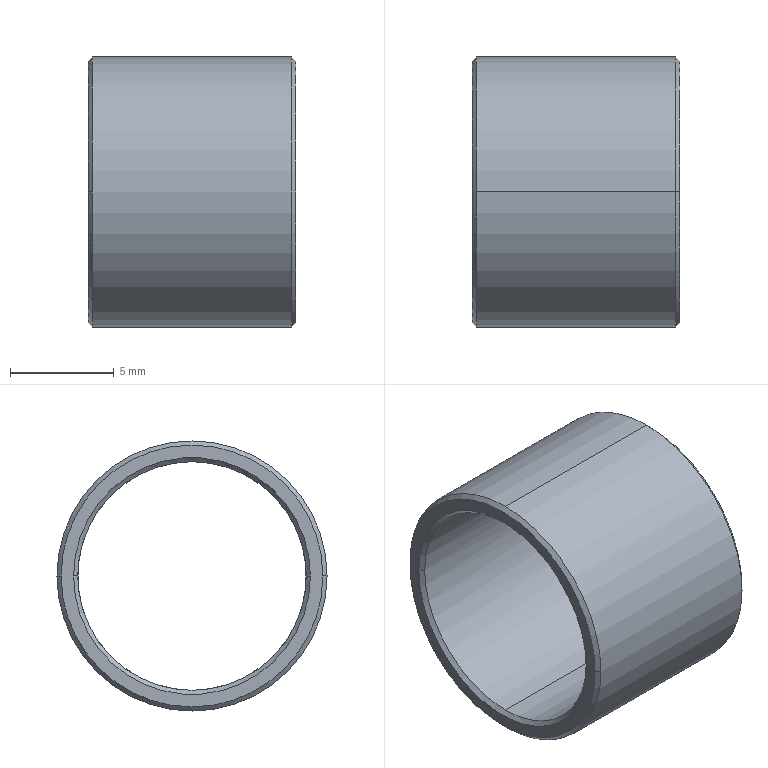Part | SolidWorks | features BaseBody 1 | 1 solid | 14 faces | box 10 x 13 x 13 mm | volume 373.975 mm3 | cone 8 | cylinder 4 | plane 2 | commonest cylinder face diameters 11 x2 13 x2
STEP:
#1=CARTESIAN_POINT('',(9.8,0.,6.5));
#2=VERTEX_POINT('',#1);
#3=CARTESIAN_POINT('',(9.8,0.,-6.5));
#4=VERTEX_POINT('',#3);
#5=CARTESIAN_POINT('',(9.8,0.,0.));
#6=DIRECTION('',(-1.,0.,0.));
#7=DIRECTION('',(0.,0.,1.));
#8=AXIS2_PLACEMENT_3D('',#5,#6,#7);
#9=CIRCLE('',#8,6.5);
#10=EDGE_CURVE('',#2,#4,#9,.T.);
#11=ORIENTED_EDGE('',*,*,#10,.T.);
#12=CARTESIAN_POINT('',(0.2,0.,-6.5));
#13=VERTEX_POINT('',#12);
#14=CARTESIAN_POINT('',(5.,0.,-6.5));
#15=DIRECTION('',(-1.,0.,0.));
#16=VECTOR('',#15,1000.);
#17=LINE('',#14,#16);
#18=EDGE_CURVE('',#4,#13,#17,.T.);
#19=ORIENTED_EDGE('',*,*,#18,.T.);
#20=CARTESIAN_POINT('',(0.2,6.5,0.));
#21=VERTEX_POINT('',#20);
#22=CARTESIAN_POINT('',(0.2,0.,0.));
#23=DIRECTION('',(1.,0.,0.));
#24=DIRECTION('',(0.,0.,1.));
#25=AXIS2_PLACEMENT_3D('',#22,#23,#24);
#26=CIRCLE('',#25,6.5);
#27=EDGE_CURVE('',#13,#21,#26,.T.);
#28=ORIENTED_EDGE('',*,*,#27,.T.);
#29=CARTESIAN_POINT('',(0.2,0.,6.5));
#30=VERTEX_POINT('',#29);
#31=CARTESIAN_POINT('',(0.2,0.,0.));
#32=DIRECTION('',(1.,0.,0.));
#33=DIRECTION('',(0.,0.,1.));
#34=AXIS2_PLACEMENT_3D('',#31,#32,#33);
#35=CIRCLE('',#34,6.5);
#36=EDGE_CURVE('',#21,#30,#35,.T.);
#37=ORIENTED_EDGE('',*,*,#36,.T.);
#38=CARTESIAN_POINT('',(5.,0.,6.5));
#39=DIRECTION('',(-1.,0.,0.));
#40=VECTOR('',#39,1000.);
#41=LINE('',#38,#40);
#42=EDGE_CURVE('',#2,#30,#41,.T.);
#43=ORIENTED_EDGE('',*,*,#42,.F.);
#44=EDGE_LOOP('',(#11,#19,#28,#37,#43));
#45=FACE_OUTER_BOUND('',#44,.T.);
#46=CARTESIAN_POINT('',(5.,0.,0.));
#47=DIRECTION('',(-1.,0.,0.));
#48=DIRECTION('',(0.,0.,1.));
#49=AXIS2_PLACEMENT_3D('',#46,#47,#48);
#50=CYLINDRICAL_SURFACE('',#49,6.5);
#51=ADVANCED_FACE('',(#45),#50,.T.);
#52=CARTESIAN_POINT('',(10.,0.,6.3));
#53=VERTEX_POINT('',#52);
#54=CARTESIAN_POINT('',(10.,0.,-6.3));
#55=VERTEX_POINT('',#54);
#56=CARTESIAN_POINT('',(10.,0.,0.));
#57=DIRECTION('',(-1.,0.,0.));
#58=DIRECTION('',(0.,0.,1.));
#59=AXIS2_PLACEMENT_3D('',#56,#57,#58);
#60=CIRCLE('',#59,6.3);
#61=EDGE_CURVE('',#53,#55,#60,.T.);
#62=ORIENTED_EDGE('',*,*,#61,.T.);
#63=CARTESIAN_POINT('',(9.8,0.,-6.5));
#64=DIRECTION('',(-0.7071,0.,-0.7071));
#65=VECTOR('',#64,1000.);
#66=LINE('',#63,#65);
#67=EDGE_CURVE('',#55,#4,#66,.T.);
#68=ORIENTED_EDGE('',*,*,#67,.T.);
#69=ORIENTED_EDGE('',*,*,#10,.F.);
#70=CARTESIAN_POINT('',(9.8,0.,6.5));
#71=DIRECTION('',(-0.7071,0.,0.7071));
#72=VECTOR('',#71,1000.);
#73=LINE('',#70,#72);
#74=EDGE_CURVE('',#53,#2,#73,.T.);
#75=ORIENTED_EDGE('',*,*,#74,.F.);
#76=EDGE_LOOP('',(#62,#68,#69,#75));
#77=FACE_OUTER_BOUND('',#76,.T.);
#78=CARTESIAN_POINT('',(9.8,0.,0.));
#79=DIRECTION('',(-1.,0.,0.));
#80=DIRECTION('',(0.,0.,1.));
#81=AXIS2_PLACEMENT_3D('',#78,#79,#80);
#82=CONICAL_SURFACE('',#81,6.5,0.7854);
#83=ADVANCED_FACE('',(#77),#82,.T.);
#84=CARTESIAN_POINT('',(0.,6.3,0.));
#85=VERTEX_POINT('',#84);
#86=CARTESIAN_POINT('',(0.,-6.3,0.));
#87=VERTEX_POINT('',#86);
#88=CARTESIAN_POINT('',(0.,0.,0.));
#89=DIRECTION('',(1.,0.,0.));
#90=DIRECTION('',(0.,1.,0.));
#91=AXIS2_PLACEMENT_3D('',#88,#89,#90);
#92=CIRCLE('',#91,6.3);
#93=EDGE_CURVE('',#85,#87,#92,.T.);
#94=ORIENTED_EDGE('',*,*,#93,.T.);
#95=CARTESIAN_POINT('',(0.2,-6.5,0.));
#96=VERTEX_POINT('',#95);
#97=CARTESIAN_POINT('',(0.2,-6.5,0.));
#98=DIRECTION('',(0.7071,-0.7071,0.));
#99=VECTOR('',#98,1000.);
#100=LINE('',#97,#99);
#101=EDGE_CURVE('',#87,#96,#100,.T.);
#102=ORIENTED_EDGE('',*,*,#101,.T.);
#103=CARTESIAN_POINT('',(0.2,0.,0.));
#104=DIRECTION('',(1.,0.,0.));
#105=DIRECTION('',(0.,0.,1.));
#106=AXIS2_PLACEMENT_3D('',#103,#104,#105);
#107=CIRCLE('',#106,6.5);
#108=EDGE_CURVE('',#30,#96,#107,.T.);
#109=ORIENTED_EDGE('',*,*,#108,.F.);
#110=ORIENTED_EDGE('',*,*,#36,.F.);
#111=CARTESIAN_POINT('',(0.2,6.5,0.));
#112=DIRECTION('',(0.7071,0.7071,0.));
#113=VECTOR('',#112,1000.);
#114=LINE('',#111,#113);
#115=EDGE_CURVE('',#85,#21,#114,.T.);
#116=ORIENTED_EDGE('',*,*,#115,.F.);
#117=EDGE_LOOP('',(#94,#102,#109,#110,#116));
#118=FACE_OUTER_BOUND('',#117,.T.);
#119=CARTESIAN_POINT('',(0.2,0.,0.));
#120=DIRECTION('',(1.,0.,0.));
#121=DIRECTION('',(0.,1.,0.));
#122=AXIS2_PLACEMENT_3D('',#119,#120,#121);
#123=CONICAL_SURFACE('',#122,6.5,0.7854);
#124=ADVANCED_FACE('',(#118),#123,.T.);
#125=CARTESIAN_POINT('',(9.8,0.,5.5));
#126=VERTEX_POINT('',#125);
#127=CARTESIAN_POINT('',(9.8,0.,-5.5));
#128=VERTEX_POINT('',#127);
#129=CARTESIAN_POINT('',(9.8,0.,0.));
#130=DIRECTION('',(1.,0.,0.));
#131=DIRECTION('',(0.,-1.,0.));
#132=AXIS2_PLACEMENT_3D('',#129,#130,#131);
#133=CIRCLE('',#132,5.5);
#134=EDGE_CURVE('',#126,#128,#133,.T.);
#135=ORIENTED_EDGE('',*,*,#134,.F.);
#136=CARTESIAN_POINT('',(10.,0.,5.7));
#137=VERTEX_POINT('',#136);
#138=CARTESIAN_POINT('',(10.,0.,5.7));
#139=DIRECTION('',(0.7071,0.,0.7071));
#140=VECTOR('',#139,1000.);
#141=LINE('',#138,#140);
#142=EDGE_CURVE('',#126,#137,#141,.T.);
#143=ORIENTED_EDGE('',*,*,#142,.T.);
#144=CARTESIAN_POINT('',(10.,0.,-5.7));
#145=VERTEX_POINT('',#144);
#146=CARTESIAN_POINT('',(10.,0.,0.));
#147=DIRECTION('',(-1.,0.,0.));
#148=DIRECTION('',(0.,0.,-1.));
#149=AXIS2_PLACEMENT_3D('',#146,#147,#148);
#150=CIRCLE('',#149,5.7);
#151=EDGE_CURVE('',#145,#137,#150,.T.);
#152=ORIENTED_EDGE('',*,*,#151,.F.);
#153=CARTESIAN_POINT('',(10.,0.,-5.7));
#154=DIRECTION('',(0.7071,0.,-0.7071));
#155=VECTOR('',#154,1000.);
#156=LINE('',#153,#155);
#157=EDGE_CURVE('',#128,#145,#156,.T.);
#158=ORIENTED_EDGE('',*,*,#157,.F.);
#159=EDGE_LOOP('',(#135,#143,#152,#158));
#160=FACE_OUTER_BOUND('',#159,.T.);
#161=CARTESIAN_POINT('',(10.,0.,0.));
#162=DIRECTION('',(1.,0.,0.));
#163=DIRECTION('',(0.,0.,-1.));
#164=AXIS2_PLACEMENT_3D('',#161,#162,#163);
#165=CONICAL_SURFACE('',#164,5.7,0.7854);
#166=ADVANCED_FACE('',(#160),#165,.F.);
#167=CARTESIAN_POINT('',(0.2,5.5,0.));
#168=VERTEX_POINT('',#167);
#169=CARTESIAN_POINT('',(0.2,0.,-5.5));
#170=VERTEX_POINT('',#169);
#171=CARTESIAN_POINT('',(0.2,0.,0.));
#172=DIRECTION('',(-1.,0.,0.));
#173=DIRECTION('',(0.,-1.,0.));
#174=AXIS2_PLACEMENT_3D('',#171,#172,#173);
#175=CIRCLE('',#174,5.5);
#176=EDGE_CURVE('',#168,#170,#175,.T.);
#177=ORIENTED_EDGE('',*,*,#176,.F.);
#178=CARTESIAN_POINT('',(0.,5.7,0.));
#179=VERTEX_POINT('',#178);
#180=CARTESIAN_POINT('',(0.,5.7,0.));
#181=DIRECTION('',(-0.7071,0.7071,0.));
#182=VECTOR('',#181,1000.);
#183=LINE('',#180,#182);
#184=EDGE_CURVE('',#168,#179,#183,.T.);
#185=ORIENTED_EDGE('',*,*,#184,.T.);
#186=CARTESIAN_POINT('',(0.,-5.7,0.));
#187=VERTEX_POINT('',#186);
#188=CARTESIAN_POINT('',(0.,0.,0.));
#189=DIRECTION('',(1.,0.,0.));
#190=DIRECTION('',(0.,-1.,0.));
#191=AXIS2_PLACEMENT_3D('',#188,#189,#190);
#192=CIRCLE('',#191,5.7);
#193=EDGE_CURVE('',#187,#179,#192,.T.);
#194=ORIENTED_EDGE('',*,*,#193,.F.);
#195=CARTESIAN_POINT('',(0.2,-5.5,0.));
#196=VERTEX_POINT('',#195);
#197=CARTESIAN_POINT('',(0.,-5.7,0.));
#198=DIRECTION('',(-0.7071,-0.7071,0.));
#199=VECTOR('',#198,1000.);
#200=LINE('',#197,#199);
#201=EDGE_CURVE('',#196,#187,#200,.T.);
#202=ORIENTED_EDGE('',*,*,#201,.F.);
#203=CARTESIAN_POINT('',(0.2,0.,0.));
#204=DIRECTION('',(-1.,0.,0.));
#205=DIRECTION('',(0.,-1.,0.));
#206=AXIS2_PLACEMENT_3D('',#203,#204,#205);
#207=CIRCLE('',#206,5.5);
#208=EDGE_CURVE('',#170,#196,#207,.T.);
#209=ORIENTED_EDGE('',*,*,#208,.F.);
#210=EDGE_LOOP('',(#177,#185,#194,#202,#209));
#211=FACE_OUTER_BOUND('',#210,.T.);
#212=CARTESIAN_POINT('',(0.,0.,0.));
#213=DIRECTION('',(-1.,0.,0.));
#214=DIRECTION('',(0.,-1.,0.));
#215=AXIS2_PLACEMENT_3D('',#212,#213,#214);
#216=CONICAL_SURFACE('',#215,5.7,0.7854);
#217=ADVANCED_FACE('',(#211),#216,.F.);
#218=ORIENTED_EDGE('',*,*,#134,.T.);
#219=CARTESIAN_POINT('',(5.,0.,-5.5));
#220=DIRECTION('',(-1.,0.,0.));
#221=VECTOR('',#220,1000.);
#222=LINE('',#219,#221);
#223=EDGE_CURVE('',#128,#170,#222,.T.);
#224=ORIENTED_EDGE('',*,*,#223,.T.);
#225=ORIENTED_EDGE('',*,*,#208,.T.);
#226=CARTESIAN_POINT('',(0.2,0.,5.5));
#227=VERTEX_POINT('',#226);
#228=CARTESIAN_POINT('',(0.2,0.,0.));
#229=DIRECTION('',(-1.,0.,0.));
#230=DIRECTION('',(0.,-1.,0.));
#231=AXIS2_PLACEMENT_3D('',#228,#229,#230);
#232=CIRCLE('',#231,5.5);
#233=EDGE_CURVE('',#196,#227,#232,.T.);
#234=ORIENTED_EDGE('',*,*,#233,.T.);
#235=CARTESIAN_POINT('',(5.,0.,5.5));
#236=DIRECTION('',(-1.,0.,0.));
#237=VECTOR('',#236,1000.);
#238=LINE('',#235,#237);
#239=EDGE_CURVE('',#126,#227,#238,.T.);
#240=ORIENTED_EDGE('',*,*,#239,.F.);
#241=EDGE_LOOP('',(#218,#224,#225,#234,#240));
#242=FACE_OUTER_BOUND('',#241,.T.);
#243=CARTESIAN_POINT('',(5.,0.,0.));
#244=DIRECTION('',(-1.,0.,0.));
#245=DIRECTION('',(0.,0.,1.));
#246=AXIS2_PLACEMENT_3D('',#243,#244,#245);
#247=CYLINDRICAL_SURFACE('',#246,5.5);
#248=ADVANCED_FACE('',(#242),#247,.F.);
#249=ORIENTED_EDGE('',*,*,#18,.F.);
#250=CARTESIAN_POINT('',(9.8,0.,0.));
#251=DIRECTION('',(-1.,0.,0.));
#252=DIRECTION('',(0.,0.,1.));
#253=AXIS2_PLACEMENT_3D('',#250,#251,#252);
#254=CIRCLE('',#253,6.5);
#255=EDGE_CURVE('',#4,#2,#254,.T.);
#256=ORIENTED_EDGE('',*,*,#255,.T.);
#257=ORIENTED_EDGE('',*,*,#42,.T.);
#258=ORIENTED_EDGE('',*,*,#108,.T.);
#259=CARTESIAN_POINT('',(0.2,0.,0.));
#260=DIRECTION('',(1.,0.,0.));
#261=DIRECTION('',(0.,0.,1.));
#262=AXIS2_PLACEMENT_3D('',#259,#260,#261);
#263=CIRCLE('',#262,6.5);
#264=EDGE_CURVE('',#96,#13,#263,.T.);
#265=ORIENTED_EDGE('',*,*,#264,.T.);
#266=EDGE_LOOP('',(#249,#256,#257,#258,#265));
#267=FACE_OUTER_BOUND('',#266,.T.);
#268=CARTESIAN_POINT('',(5.,0.,0.));
#269=DIRECTION('',(-1.,0.,0.));
#270=DIRECTION('',(0.,0.,1.));
#271=AXIS2_PLACEMENT_3D('',#268,#269,#270);
#272=CYLINDRICAL_SURFACE('',#271,6.5);
#273=ADVANCED_FACE('',(#267),#272,.T.);
#274=ORIENTED_EDGE('',*,*,#67,.F.);
#275=CARTESIAN_POINT('',(10.,0.,0.));
#276=DIRECTION('',(-1.,0.,0.));
#277=DIRECTION('',(0.,0.,1.));
#278=AXIS2_PLACEMENT_3D('',#275,#276,#277);
#279=CIRCLE('',#278,6.3);
#280=EDGE_CURVE('',#55,#53,#279,.T.);
#281=ORIENTED_EDGE('',*,*,#280,.T.);
#282=ORIENTED_EDGE('',*,*,#74,.T.);
#283=ORIENTED_EDGE('',*,*,#255,.F.);
#284=EDGE_LOOP('',(#274,#281,#282,#283));
#285=FACE_OUTER_BOUND('',#284,.T.);
#286=CARTESIAN_POINT('',(9.8,0.,0.));
#287=DIRECTION('',(-1.,0.,0.));
#288=DIRECTION('',(0.,0.,1.));
#289=AXIS2_PLACEMENT_3D('',#286,#287,#288);
#290=CONICAL_SURFACE('',#289,6.5,0.7854);
#291=ADVANCED_FACE('',(#285),#290,.T.);
#292=ORIENTED_EDGE('',*,*,#101,.F.);
#293=CARTESIAN_POINT('',(0.,0.,0.));
#294=DIRECTION('',(1.,0.,0.));
#295=DIRECTION('',(0.,1.,0.));
#296=AXIS2_PLACEMENT_3D('',#293,#294,#295);
#297=CIRCLE('',#296,6.3);
#298=EDGE_CURVE('',#87,#85,#297,.T.);
#299=ORIENTED_EDGE('',*,*,#298,.T.);
#300=ORIENTED_EDGE('',*,*,#115,.T.);
#301=ORIENTED_EDGE('',*,*,#27,.F.);
#302=ORIENTED_EDGE('',*,*,#264,.F.);
#303=EDGE_LOOP('',(#292,#299,#300,#301,#302));
#304=FACE_OUTER_BOUND('',#303,.T.);
#305=CARTESIAN_POINT('',(0.2,0.,0.));
#306=DIRECTION('',(1.,0.,0.));
#307=DIRECTION('',(0.,1.,0.));
#308=AXIS2_PLACEMENT_3D('',#305,#306,#307);
#309=CONICAL_SURFACE('',#308,6.5,0.7854);
#310=ADVANCED_FACE('',(#304),#309,.T.);
#311=ORIENTED_EDGE('',*,*,#151,.T.);
#312=CARTESIAN_POINT('',(10.,0.,0.));
#313=DIRECTION('',(-1.,0.,0.));
#314=DIRECTION('',(0.,0.,-1.));
#315=AXIS2_PLACEMENT_3D('',#312,#313,#314);
#316=CIRCLE('',#315,5.7);
#317=EDGE_CURVE('',#137,#145,#316,.T.);
#318=ORIENTED_EDGE('',*,*,#317,.T.);
#319=EDGE_LOOP('',(#311,#318));
#320=FACE_BOUND('',#319,.T.);
#321=ORIENTED_EDGE('',*,*,#61,.F.);
#322=ORIENTED_EDGE('',*,*,#280,.F.);
#323=EDGE_LOOP('',(#321,#322));
#324=FACE_OUTER_BOUND('',#323,.T.);
#325=CARTESIAN_POINT('',(10.,-3.25,0.));
#326=DIRECTION('',(1.,0.,0.));
#327=DIRECTION('',(0.,0.,-1.));
#328=AXIS2_PLACEMENT_3D('',#325,#326,#327);
#329=PLANE('',#328);
#330=ADVANCED_FACE('',(#320,#324),#329,.T.);
#331=ORIENTED_EDGE('',*,*,#93,.F.);
#332=ORIENTED_EDGE('',*,*,#298,.F.);
#333=EDGE_LOOP('',(#331,#332));
#334=FACE_OUTER_BOUND('',#333,.T.);
#335=ORIENTED_EDGE('',*,*,#193,.T.);
#336=CARTESIAN_POINT('',(0.,0.,0.));
#337=DIRECTION('',(1.,0.,0.));
#338=DIRECTION('',(0.,-1.,0.));
#339=AXIS2_PLACEMENT_3D('',#336,#337,#338);
#340=CIRCLE('',#339,5.7);
#341=EDGE_CURVE('',#179,#187,#340,.T.);
#342=ORIENTED_EDGE('',*,*,#341,.T.);
#343=EDGE_LOOP('',(#335,#342));
#344=FACE_BOUND('',#343,.T.);
#345=CARTESIAN_POINT('',(0.,-3.25,0.));
#346=DIRECTION('',(-1.,0.,0.));
#347=DIRECTION('',(0.,0.,1.));
#348=AXIS2_PLACEMENT_3D('',#345,#346,#347);
#349=PLANE('',#348);
#350=ADVANCED_FACE('',(#334,#344),#349,.T.);
#351=ORIENTED_EDGE('',*,*,#142,.F.);
#352=CARTESIAN_POINT('',(9.8,0.,0.));
#353=DIRECTION('',(1.,0.,0.));
#354=DIRECTION('',(0.,-1.,0.));
#355=AXIS2_PLACEMENT_3D('',#352,#353,#354);
#356=CIRCLE('',#355,5.5);
#357=EDGE_CURVE('',#128,#126,#356,.T.);
#358=ORIENTED_EDGE('',*,*,#357,.F.);
#359=ORIENTED_EDGE('',*,*,#157,.T.);
#360=ORIENTED_EDGE('',*,*,#317,.F.);
#361=EDGE_LOOP('',(#351,#358,#359,#360));
#362=FACE_OUTER_BOUND('',#361,.T.);
#363=CARTESIAN_POINT('',(10.,0.,0.));
#364=DIRECTION('',(1.,0.,0.));
#365=DIRECTION('',(0.,0.,-1.));
#366=AXIS2_PLACEMENT_3D('',#363,#364,#365);
#367=CONICAL_SURFACE('',#366,5.7,0.7854);
#368=ADVANCED_FACE('',(#362),#367,.F.);
#369=ORIENTED_EDGE('',*,*,#184,.F.);
#370=CARTESIAN_POINT('',(0.2,0.,0.));
#371=DIRECTION('',(-1.,0.,0.));
#372=DIRECTION('',(0.,-1.,0.));
#373=AXIS2_PLACEMENT_3D('',#370,#371,#372);
#374=CIRCLE('',#373,5.5);
#375=EDGE_CURVE('',#227,#168,#374,.T.);
#376=ORIENTED_EDGE('',*,*,#375,.F.);
#377=ORIENTED_EDGE('',*,*,#233,.F.);
#378=ORIENTED_EDGE('',*,*,#201,.T.);
#379=ORIENTED_EDGE('',*,*,#341,.F.);
#380=EDGE_LOOP('',(#369,#376,#377,#378,#379));
#381=FACE_OUTER_BOUND('',#380,.T.);
#382=CARTESIAN_POINT('',(0.,0.,0.));
#383=DIRECTION('',(-1.,0.,0.));
#384=DIRECTION('',(0.,-1.,0.));
#385=AXIS2_PLACEMENT_3D('',#382,#383,#384);
#386=CONICAL_SURFACE('',#385,5.7,0.7854);
#387=ADVANCED_FACE('',(#381),#386,.F.);
#388=ORIENTED_EDGE('',*,*,#223,.F.);
#389=ORIENTED_EDGE('',*,*,#357,.T.);
#390=ORIENTED_EDGE('',*,*,#239,.T.);
#391=ORIENTED_EDGE('',*,*,#375,.T.);
#392=ORIENTED_EDGE('',*,*,#176,.T.);
#393=EDGE_LOOP('',(#388,#389,#390,#391,#392));
#394=FACE_OUTER_BOUND('',#393,.T.);
#395=CARTESIAN_POINT('',(5.,0.,0.));
#396=DIRECTION('',(-1.,0.,0.));
#397=DIRECTION('',(0.,0.,1.));
#398=AXIS2_PLACEMENT_3D('',#395,#396,#397);
#399=CYLINDRICAL_SURFACE('',#398,5.5);
#400=ADVANCED_FACE('',(#394),#399,.F.);
#401=CLOSED_SHELL('',(#51,#83,#124,#166,#217,#248,#273,#291,#310,#330,#350,#368,#387,#400));
#402=MANIFOLD_SOLID_BREP('',#401);
#403=CARTESIAN_POINT('',(0.,0.,0.));
#404=DIRECTION('',(0.,0.,1.));
#405=DIRECTION('',(1.,0.,0.));
#406=AXIS2_PLACEMENT_3D('',#403,#404,#405);
#407=(LENGTH_UNIT()NAMED_UNIT(*)SI_UNIT(.MILLI.,.METRE.));
#408=UNCERTAINTY_MEASURE_WITH_UNIT(LENGTH_MEASURE(0.00001),#407,'','');
#409=(NAMED_UNIT(*)PLANE_ANGLE_UNIT()SI_UNIT($,.RADIAN.));
#410=(NAMED_UNIT(*)SI_UNIT($,.STERADIAN.)SOLID_ANGLE_UNIT());
#411=(GEOMETRIC_REPRESENTATION_CONTEXT(3)GLOBAL_UNCERTAINTY_ASSIGNED_CONTEXT((#408))GLOBAL_UNIT_ASSIGNED_CONTEXT((#407,#409,#410))REPRESENTATION_CONTEXT('',''));
#412=ADVANCED_BREP_SHAPE_REPRESENTATION('',(#402,#406),#411);